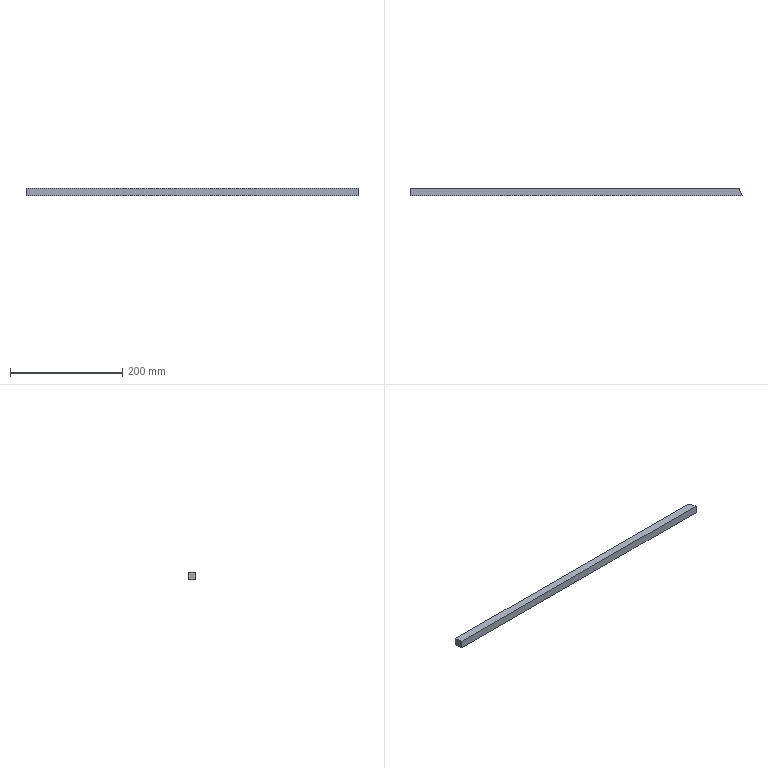Part | NX | features solid 2 | 1 solid | 6 faces | box 591.317 x 14 x 14 mm | volume 115399 mm3 | plane 6
STEP:
#1=CARTESIAN_POINT('',(-285.,119.,-5.));
#2=VERTEX_POINT('',#1);
#3=CARTESIAN_POINT('',(301.221,119.,-5.));
#4=VERTEX_POINT('',#3);
#5=CARTESIAN_POINT('',(-285.,119.,-5.));
#6=DIRECTION('',(1.,0.,0.));
#7=VECTOR('',#6,1000.);
#8=LINE('',#5,#7);
#9=EDGE_CURVE('',#2,#4,#8,.T.);
#10=ORIENTED_EDGE('',*,*,#9,.F.);
#11=CARTESIAN_POINT('',(-285.,119.,9.));
#12=VERTEX_POINT('',#11);
#13=CARTESIAN_POINT('',(-285.,119.,9.));
#14=DIRECTION('',(0.,0.,-1.));
#15=VECTOR('',#14,1000.);
#16=LINE('',#13,#15);
#17=EDGE_CURVE('',#12,#2,#16,.T.);
#18=ORIENTED_EDGE('',*,*,#17,.F.);
#19=CARTESIAN_POINT('',(301.221,119.,9.));
#20=VERTEX_POINT('',#19);
#21=CARTESIAN_POINT('',(-285.,119.,9.));
#22=DIRECTION('',(1.,0.,0.));
#23=VECTOR('',#22,1000.);
#24=LINE('',#21,#23);
#25=EDGE_CURVE('',#12,#20,#24,.T.);
#26=ORIENTED_EDGE('',*,*,#25,.T.);
#27=CARTESIAN_POINT('',(301.221,119.,9.));
#28=DIRECTION('',(0.,0.,-1.));
#29=VECTOR('',#28,1000.);
#30=LINE('',#27,#29);
#31=EDGE_CURVE('',#20,#4,#30,.T.);
#32=ORIENTED_EDGE('',*,*,#31,.T.);
#33=EDGE_LOOP('',(#10,#18,#26,#32));
#34=FACE_BOUND('',#33,.T.);
#35=CARTESIAN_POINT('',(-285.,119.,9.));
#36=DIRECTION('',(0.,1.,0.));
#37=DIRECTION('',(-1.,0.,0.));
#38=AXIS2_PLACEMENT_3D('',#35,#36,#37);
#39=PLANE('',#38);
#40=ADVANCED_FACE('',(#34),#39,.T.);
#41=CARTESIAN_POINT('',(-285.,105.,-5.));
#42=VERTEX_POINT('',#41);
#43=CARTESIAN_POINT('',(-285.,150.,-5.));
#44=DIRECTION('',(0.,-1.,0.));
#45=VECTOR('',#44,1000.);
#46=LINE('',#43,#45);
#47=EDGE_CURVE('',#2,#42,#46,.T.);
#48=ORIENTED_EDGE('',*,*,#47,.T.);
#49=CARTESIAN_POINT('',(-285.,105.,9.));
#50=VERTEX_POINT('',#49);
#51=CARTESIAN_POINT('',(-285.,105.,9.));
#52=DIRECTION('',(0.,0.,-1.));
#53=VECTOR('',#52,1000.);
#54=LINE('',#51,#53);
#55=EDGE_CURVE('',#50,#42,#54,.T.);
#56=ORIENTED_EDGE('',*,*,#55,.F.);
#57=CARTESIAN_POINT('',(-285.,150.,9.));
#58=DIRECTION('',(0.,-1.,0.));
#59=VECTOR('',#58,1000.);
#60=LINE('',#57,#59);
#61=EDGE_CURVE('',#12,#50,#60,.T.);
#62=ORIENTED_EDGE('',*,*,#61,.F.);
#63=ORIENTED_EDGE('',*,*,#17,.T.);
#64=EDGE_LOOP('',(#48,#56,#62,#63));
#65=FACE_BOUND('',#64,.T.);
#66=CARTESIAN_POINT('',(-285.,150.,9.));
#67=DIRECTION('',(1.,0.,0.));
#68=DIRECTION('',(0.,0.,-1.));
#69=AXIS2_PLACEMENT_3D('',#66,#67,#68);
#70=PLANE('',#69);
#71=ADVANCED_FACE('',(#65),#70,.F.);
#72=CARTESIAN_POINT('',(306.317,105.,-5.));
#73=VERTEX_POINT('',#72);
#74=CARTESIAN_POINT('',(-285.,105.,-5.));
#75=DIRECTION('',(1.,0.,0.));
#76=VECTOR('',#75,1000.);
#77=LINE('',#74,#76);
#78=EDGE_CURVE('',#42,#73,#77,.T.);
#79=ORIENTED_EDGE('',*,*,#78,.T.);
#80=CARTESIAN_POINT('',(306.317,105.,9.));
#81=VERTEX_POINT('',#80);
#82=CARTESIAN_POINT('',(306.317,105.,9.));
#83=DIRECTION('',(0.,0.,-1.));
#84=VECTOR('',#83,1000.);
#85=LINE('',#82,#84);
#86=EDGE_CURVE('',#81,#73,#85,.T.);
#87=ORIENTED_EDGE('',*,*,#86,.F.);
#88=CARTESIAN_POINT('',(-285.,105.,9.));
#89=DIRECTION('',(1.,0.,0.));
#90=VECTOR('',#89,1000.);
#91=LINE('',#88,#90);
#92=EDGE_CURVE('',#50,#81,#91,.T.);
#93=ORIENTED_EDGE('',*,*,#92,.F.);
#94=ORIENTED_EDGE('',*,*,#55,.T.);
#95=EDGE_LOOP('',(#79,#87,#93,#94));
#96=FACE_BOUND('',#95,.T.);
#97=CARTESIAN_POINT('',(-285.,105.,9.));
#98=DIRECTION('',(0.,1.,0.));
#99=DIRECTION('',(-1.,0.,0.));
#100=AXIS2_PLACEMENT_3D('',#97,#98,#99);
#101=PLANE('',#100);
#102=ADVANCED_FACE('',(#96),#101,.F.);
#103=CARTESIAN_POINT('',(300.,122.355,-5.));
#104=DIRECTION('',(0.342,-0.9397,0.));
#105=VECTOR('',#104,1000.);
#106=LINE('',#103,#105);
#107=EDGE_CURVE('',#4,#73,#106,.T.);
#108=ORIENTED_EDGE('',*,*,#107,.F.);
#109=ORIENTED_EDGE('',*,*,#31,.F.);
#110=CARTESIAN_POINT('',(300.,122.355,9.));
#111=DIRECTION('',(0.342,-0.9397,0.));
#112=VECTOR('',#111,1000.);
#113=LINE('',#110,#112);
#114=EDGE_CURVE('',#20,#81,#113,.T.);
#115=ORIENTED_EDGE('',*,*,#114,.T.);
#116=ORIENTED_EDGE('',*,*,#86,.T.);
#117=EDGE_LOOP('',(#108,#109,#115,#116));
#118=FACE_BOUND('',#117,.T.);
#119=CARTESIAN_POINT('',(300.,122.355,9.));
#120=DIRECTION('',(0.9397,0.342,0.));
#121=DIRECTION('',(-0.342,0.9397,0.));
#122=AXIS2_PLACEMENT_3D('',#119,#120,#121);
#123=PLANE('',#122);
#124=ADVANCED_FACE('',(#118),#123,.T.);
#125=ORIENTED_EDGE('',*,*,#25,.F.);
#126=ORIENTED_EDGE('',*,*,#61,.T.);
#127=ORIENTED_EDGE('',*,*,#92,.T.);
#128=ORIENTED_EDGE('',*,*,#114,.F.);
#129=EDGE_LOOP('',(#125,#126,#127,#128));
#130=FACE_BOUND('',#129,.T.);
#131=CARTESIAN_POINT('',(-138.75,124.089,9.));
#132=DIRECTION('',(0.,0.,1.));
#133=DIRECTION('',(1.,0.,0.));
#134=AXIS2_PLACEMENT_3D('',#131,#132,#133);
#135=PLANE('',#134);
#136=ADVANCED_FACE('',(#130),#135,.T.);
#137=ORIENTED_EDGE('',*,*,#9,.T.);
#138=ORIENTED_EDGE('',*,*,#107,.T.);
#139=ORIENTED_EDGE('',*,*,#78,.F.);
#140=ORIENTED_EDGE('',*,*,#47,.F.);
#141=EDGE_LOOP('',(#137,#138,#139,#140));
#142=FACE_BOUND('',#141,.T.);
#143=CARTESIAN_POINT('',(-138.75,124.089,-5.));
#144=DIRECTION('',(0.,0.,1.));
#145=DIRECTION('',(1.,0.,0.));
#146=AXIS2_PLACEMENT_3D('',#143,#144,#145);
#147=PLANE('',#146);
#148=ADVANCED_FACE('',(#142),#147,.F.);
#149=CLOSED_SHELL('',(#40,#71,#102,#124,#136,#148));
#150=MANIFOLD_SOLID_BREP('',#149);
#151=(LENGTH_UNIT()NAMED_UNIT(*)SI_UNIT(.MILLI.,.METRE.));
#152=UNCERTAINTY_MEASURE_WITH_UNIT(LENGTH_MEASURE(0.00001),#151,'','');
#153=(NAMED_UNIT(*)PLANE_ANGLE_UNIT()SI_UNIT($,.RADIAN.));
#154=(NAMED_UNIT(*)SI_UNIT($,.STERADIAN.)SOLID_ANGLE_UNIT());
#155=(GEOMETRIC_REPRESENTATION_CONTEXT(3)GLOBAL_UNCERTAINTY_ASSIGNED_CONTEXT((#152))GLOBAL_UNIT_ASSIGNED_CONTEXT((#151,#153,#154))REPRESENTATION_CONTEXT('',''));
#156=ADVANCED_BREP_SHAPE_REPRESENTATION('',(#150),#155);